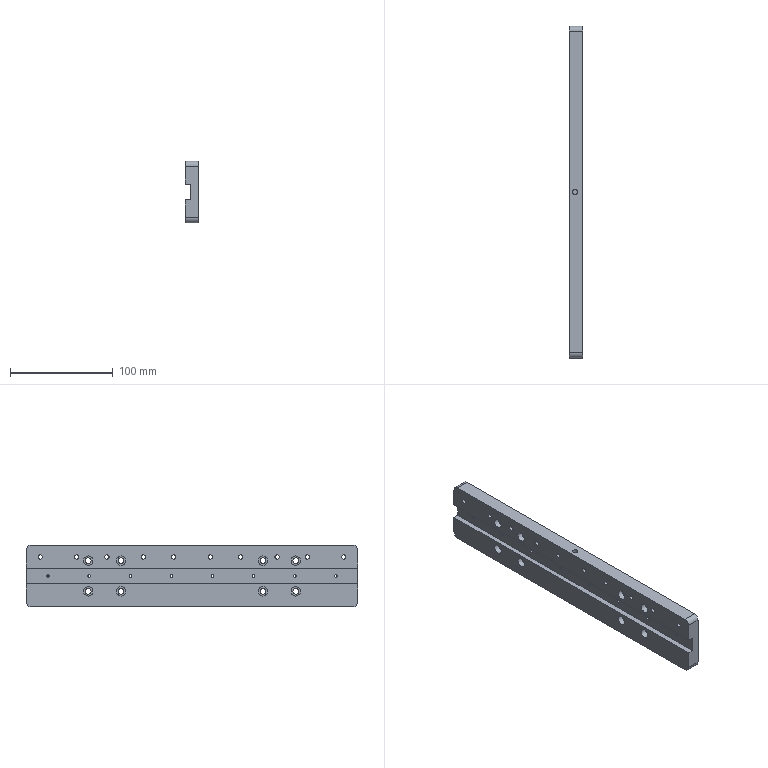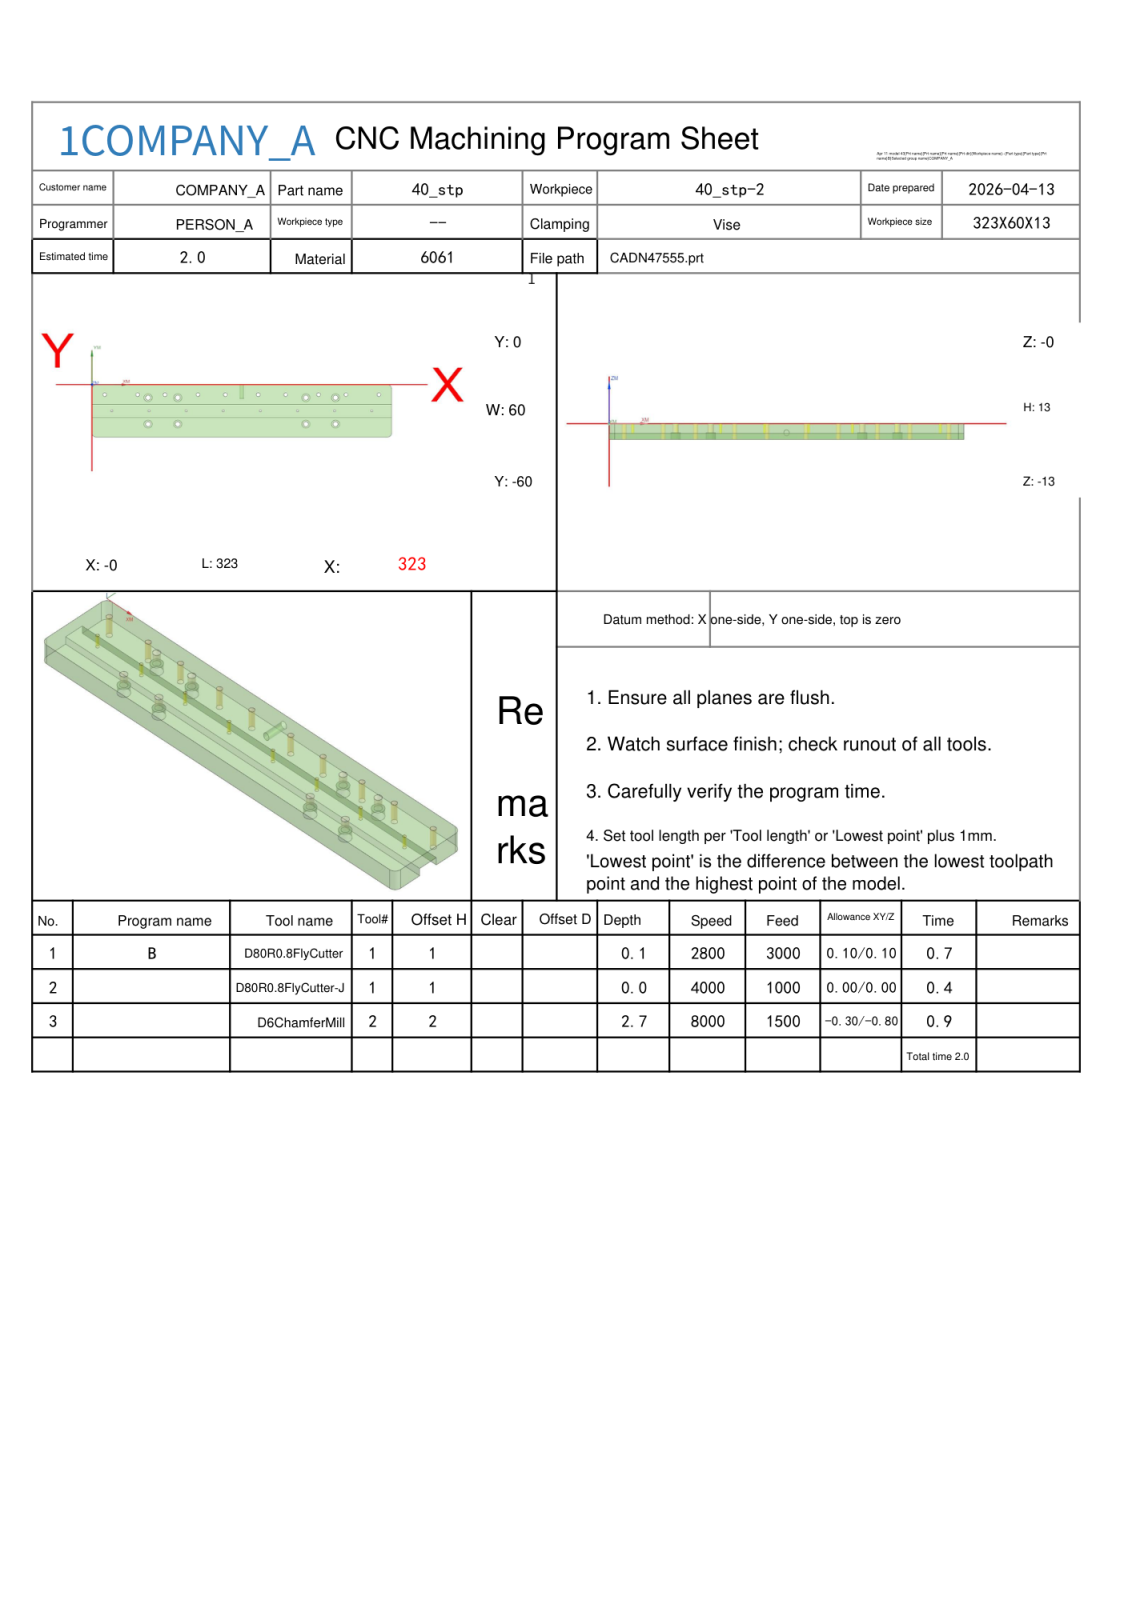NC program | NX | posted by the shop | part box 13 x 323 x 60 mm
Whole program:
%
O0001
(Machine time: 2.59 MIN)
(===Total Tool:2===)
(T1=D80R0.8 FlyCutter D=80.  R=0.8  D-  H01 Z=0.    )
(T2=D6ChamferMill   D=6.   R=0.   D-  H02 Z=-2.7  )
G80 G90 G17 G49 G40
G91 G28 Z0
M01
N1 T01 M06
(D80R0.8 FlyCutter  D=80. R=0.8 H=01 ce=0.10 di=0.10)
G00 G90 G54 X-52.097 Y-32.749 M03 S2800
G43 H01 Z20.
M08
Z3.525
G01 Z1.525 F3000.
X-40.097 Y-32.594
X363.097 Y-27.406
X375.097 Y-27.251
Z3.525
G00 X-52.097 Y-32.749
Z3.05
G01 Z1.05
X-40.097 Y-32.594
X363.097 Y-27.406
X375.097 Y-27.251
Z3.05
G00 X-52.097 Y-32.749
Z2.575
G01 Z.575
X-40.097 Y-32.594
X363.097 Y-27.406
X375.097 Y-27.251
Z2.575
G00 X-52.097 Y-32.749
Z2.1
G01 Z.1
X-40.097 Y-32.594
X363.097 Y-27.406
X375.097 Y-27.251
Z2.1
G00 Z20.
G91 G28 Z0.0
M05
M09
G91 G28 Z0.0
M01
N2 T01 M06
(D80R0.8 FlyCutter-J  D=80. R=0.8 H=01 ce=0.00 di=0.00)
G00 G90 G54 X-51.999 Y-32.75 M03 S4000
G43 H01 Z20.
M08
Z2.
G01 Z0.0 F1000.
X-39.999 Y-32.596
X362.999 Y-27.404
X374.999 Y-27.25
Z2.
G00 Z20.
G91 G28 Z0.0
M05
M09
G91 G28 Z0.0
M01
N3 T02 M06
(D6ChamferMill  D=6. R=0. H=02 ce=0.00 di=0.00)
G00 G90 G54 X301.5 Y-30. M03 S8000
G43 H02 Z20.
M08
G98 G81 X301.5 Y-30. Z-1.75 R3. F1000.
X261.5
X221.5
X181.5
X141.5
X101.5
X61.5
X21.5
G80
G00 Z20.
G00 G90 X13.75 Y-11.5 M03 S8000
Z20.
G98 G81 X13.75 Y-11.5 Z-2.7 R3. F1000.
X49.25
X78.75
X114.25
X143.75
X179.25
X208.75
X244.25
X273.75
X309.25
G80
G00 Z20.
G00 G90 X61.147 Y-14.935 M03 S8000
Z20.
Z-.9
G01 Z-1.4 F1200.
X62. Y-14.85
G03 X60.5 Y-13.35 I-1.5 J0.0
X58.85 Y-15. I0.0 J-1.65
X60.5 Y-16.65 I1.65 J0.0
X62.15 Y-15. I0.0 J1.65
X60.5 Y-13.35 I-1.65 J0.0
X59. Y-14.85 I0.0 J-1.5
G01 X59.853 Y-14.935
Z-.9
G00 Z20.
X61.147 Y-44.935
Z-.9
G01 Z-1.4
X62. Y-44.85
G03 X60.5 Y-43.35 I-1.5 J0.0
X58.85 Y-45. I0.0 J-1.65
X60.5 Y-46.65 I1.65 J0.0
X62.15 Y-45. I0.0 J1.65
X60.5 Y-43.35 I-1.65 J0.0
X59. Y-44.85 I0.0 J-1.5
G01 X59.853 Y-44.935
Z-.9
G00 Z20.
X93.147
Z-.9
G01 Z-1.4
X94. Y-44.85
G03 X92.5 Y-43.35 I-1.5 J0.0
X90.85 Y-45. I0.0 J-1.65
X92.5 Y-46.65 I1.65 J0.0
X94.15 Y-45. I0.0 J1.65
X92.5 Y-43.35 I-1.65 J0.0
X91. Y-44.85 I0.0 J-1.5
G01 X91.853 Y-44.935
Z-.9
G00 Z20.
X93.147 Y-14.935
Z-.9
G01 Z-1.4
X94. Y-14.85
G03 X92.5 Y-13.35 I-1.5 J0.0
X90.85 Y-15. I0.0 J-1.65
X92.5 Y-16.65 I1.65 J0.0
X94.15 Y-15. I0.0 J1.65
X92.5 Y-13.35 I-1.65 J0.0
X91. Y-14.85 I0.0 J-1.5
G01 X91.853 Y-14.935
Z-.9
G00 Z20.
X231.147
Z-.9
G01 Z-1.4
X232. Y-14.85
G03 X230.5 Y-13.35 I-1.5 J0.0
X228.85 Y-15. I0.0 J-1.65
X230.5 Y-16.65 I1.65 J0.0
X232.15 Y-15. I0.0 J1.65
X230.5 Y-13.35 I-1.65 J0.0
X229. Y-14.85 I0.0 J-1.5
G01 X229.853 Y-14.935
Z-.9
G00 Z20.
X231.147 Y-44.935
Z-.9
G01 Z-1.4
X232. Y-44.85
G03 X230.5 Y-43.35 I-1.5 J0.0
X228.85 Y-45. I0.0 J-1.65
X230.5 Y-46.65 I1.65 J0.0
X232.15 Y-45. I0.0 J1.65
X230.5 Y-43.35 I-1.65 J0.0
X229. Y-44.85 I0.0 J-1.5
G01 X229.853 Y-44.935
Z-.9
G00 Z20.
X263.147
Z-.9
G01 Z-1.4
X264. Y-44.85
G03 X262.5 Y-43.35 I-1.5 J0.0
X260.85 Y-45. I0.0 J-1.65
X262.5 Y-46.65 I1.65 J0.0
X264.15 Y-45. I0.0 J1.65
X262.5 Y-43.35 I-1.65 J0.0
X261. Y-44.85 I0.0 J-1.5
G01 X261.853 Y-44.935
Z-.9
G00 Z20.
X263.147 Y-14.935
Z-.9
G01 Z-1.4
X264. Y-14.85
G03 X262.5 Y-13.35 I-1.5 J0.0
X260.85 Y-15. I0.0 J-1.65
X262.5 Y-16.65 I1.65 J0.0
X264.15 Y-15. I0.0 J1.65
X262.5 Y-13.35 I-1.65 J0.0
X261. Y-14.85 I0.0 J-1.5
G01 X261.853 Y-14.935
Z-.9
G00 Z20.
G00 G90 X-.7 Y-5.661 M03 S7000
Z20.
Z2.5
G01 Y-4.815 Z2.192 F1500.
X-.661 Y-4.312 Z2.008
X-.578 Y-3.813 Z1.825
X-.451 Y-3.325 Z1.641
X-.282 Y-2.849 Z1.457
X-.071 Y-2.39 Z1.273
X.18 Y-1.952 Z1.089
X.469 Y-1.537 Z.905
X.793 Y-1.15 Z.722
X1.15 Y-.793 Z.538
X1.537 Y-.469 Z.354
X1.952 Y-.18 Z.17
X2.39 Y.071 Z-.014
X2.849 Y.282 Z-.197
X3.325 Y.451 Z-.381
X3.813 Y.578 Z-.565
X4.312 Y.661 Z-.749
X4.815 Y.7 Z-.933
X5. Z-1.
X318.
G02 X323.7 Y-5. I0.0 J-5.7
G01 Y-55.
G02 X318. Y-60.7 I-5.7 J0.0
G01 X5.
G02 X-.7 Y-55. I0.0 J5.7
G01 Y-5.
G02 X5. Y.7 I5.7 J0.0
G01 X5.5
Z1.5
G00 Z20.
M05
M09
G91 G28 Z0.0
G91 G28 Y0.0
M30
%